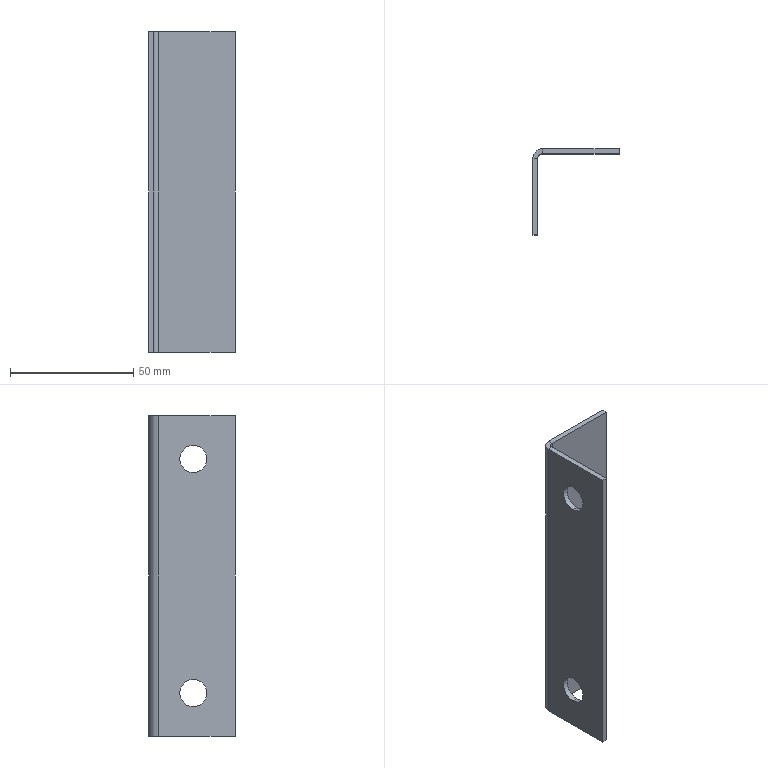Part | SolidWorks | features FlatPattern 1, ICE 1, SMBaseFlange 1, SheetMetal 1 | 1 solid | 18 faces | box 35 x 35 x 130 mm | volume 16965 mm3 | plane 12 | cylinder 6 | commonest cylinder face diameters 11 x4 4 x1 8 x1
STEP:
#1=CARTESIAN_POINT('',(0.,17.,107.));
#2=VERTEX_POINT('',#1);
#3=CARTESIAN_POINT('',(0.,17.,118.));
#4=VERTEX_POINT('',#3);
#5=CARTESIAN_POINT('',(0.,17.,112.5));
#6=DIRECTION('',(-1.,0.,0.));
#7=DIRECTION('',(0.,0.,1.));
#8=AXIS2_PLACEMENT_3D('',#5,#6,#7);
#9=CIRCLE('',#8,5.5);
#10=EDGE_CURVE('',#2,#4,#9,.T.);
#11=ORIENTED_EDGE('',*,*,#10,.T.);
#12=CARTESIAN_POINT('',(2.,17.,118.));
#13=VERTEX_POINT('',#12);
#14=CARTESIAN_POINT('',(-8.,17.,118.));
#15=DIRECTION('',(1.,0.,0.));
#16=VECTOR('',#15,1000.);
#17=LINE('',#14,#16);
#18=EDGE_CURVE('',#4,#13,#17,.T.);
#19=ORIENTED_EDGE('',*,*,#18,.T.);
#20=CARTESIAN_POINT('',(2.,17.,107.));
#21=VERTEX_POINT('',#20);
#22=CARTESIAN_POINT('',(2.,17.,112.5));
#23=DIRECTION('',(1.,0.,0.));
#24=DIRECTION('',(0.,0.,-1.));
#25=AXIS2_PLACEMENT_3D('',#22,#23,#24);
#26=CIRCLE('',#25,5.5);
#27=EDGE_CURVE('',#13,#21,#26,.T.);
#28=ORIENTED_EDGE('',*,*,#27,.T.);
#29=CARTESIAN_POINT('',(-8.,17.,107.));
#30=DIRECTION('',(1.,0.,0.));
#31=VECTOR('',#30,1000.);
#32=LINE('',#29,#31);
#33=EDGE_CURVE('',#2,#21,#32,.T.);
#34=ORIENTED_EDGE('',*,*,#33,.F.);
#35=EDGE_LOOP('',(#11,#19,#28,#34));
#36=FACE_OUTER_BOUND('',#35,.T.);
#37=CARTESIAN_POINT('',(-8.,17.,112.5));
#38=DIRECTION('',(1.,0.,0.));
#39=DIRECTION('',(0.,0.,-1.));
#40=AXIS2_PLACEMENT_3D('',#37,#38,#39);
#41=CYLINDRICAL_SURFACE('',#40,5.5);
#42=ADVANCED_FACE('',(#36),#41,.F.);
#43=CARTESIAN_POINT('',(0.,17.,12.));
#44=VERTEX_POINT('',#43);
#45=CARTESIAN_POINT('',(0.,17.,23.));
#46=VERTEX_POINT('',#45);
#47=CARTESIAN_POINT('',(0.,17.,17.5));
#48=DIRECTION('',(-1.,0.,0.));
#49=DIRECTION('',(0.,0.,1.));
#50=AXIS2_PLACEMENT_3D('',#47,#48,#49);
#51=CIRCLE('',#50,5.5);
#52=EDGE_CURVE('',#44,#46,#51,.T.);
#53=ORIENTED_EDGE('',*,*,#52,.T.);
#54=CARTESIAN_POINT('',(2.,17.,23.));
#55=VERTEX_POINT('',#54);
#56=CARTESIAN_POINT('',(-8.,17.,23.));
#57=DIRECTION('',(1.,0.,0.));
#58=VECTOR('',#57,1000.);
#59=LINE('',#56,#58);
#60=EDGE_CURVE('',#46,#55,#59,.T.);
#61=ORIENTED_EDGE('',*,*,#60,.T.);
#62=CARTESIAN_POINT('',(2.,17.,12.));
#63=VERTEX_POINT('',#62);
#64=CARTESIAN_POINT('',(2.,17.,17.5));
#65=DIRECTION('',(1.,0.,0.));
#66=DIRECTION('',(0.,0.,-1.));
#67=AXIS2_PLACEMENT_3D('',#64,#65,#66);
#68=CIRCLE('',#67,5.5);
#69=EDGE_CURVE('',#55,#63,#68,.T.);
#70=ORIENTED_EDGE('',*,*,#69,.T.);
#71=CARTESIAN_POINT('',(-8.,17.,12.));
#72=DIRECTION('',(1.,0.,0.));
#73=VECTOR('',#72,1000.);
#74=LINE('',#71,#73);
#75=EDGE_CURVE('',#44,#63,#74,.T.);
#76=ORIENTED_EDGE('',*,*,#75,.F.);
#77=EDGE_LOOP('',(#53,#61,#70,#76));
#78=FACE_OUTER_BOUND('',#77,.T.);
#79=CARTESIAN_POINT('',(-8.,17.,17.5));
#80=DIRECTION('',(1.,0.,0.));
#81=DIRECTION('',(0.,0.,-1.));
#82=AXIS2_PLACEMENT_3D('',#79,#80,#81);
#83=CYLINDRICAL_SURFACE('',#82,5.5);
#84=ADVANCED_FACE('',(#78),#83,.F.);
#85=CARTESIAN_POINT('',(4.,35.,130.));
#86=VERTEX_POINT('',#85);
#87=CARTESIAN_POINT('',(4.,33.,130.));
#88=VERTEX_POINT('',#87);
#89=CARTESIAN_POINT('',(4.,35.,130.));
#90=DIRECTION('',(0.,-1.,0.));
#91=VECTOR('',#90,1000.);
#92=LINE('',#89,#91);
#93=EDGE_CURVE('',#86,#88,#92,.T.);
#94=ORIENTED_EDGE('',*,*,#93,.F.);
#95=CARTESIAN_POINT('',(0.,31.,130.));
#96=VERTEX_POINT('',#95);
#97=CARTESIAN_POINT('',(4.,31.,130.));
#98=DIRECTION('',(0.,0.,-1.));
#99=DIRECTION('',(1.,0.,0.));
#100=AXIS2_PLACEMENT_3D('',#97,#98,#99);
#101=CIRCLE('',#100,4.);
#102=EDGE_CURVE('',#96,#86,#101,.T.);
#103=ORIENTED_EDGE('',*,*,#102,.F.);
#104=CARTESIAN_POINT('',(2.,31.,130.));
#105=VERTEX_POINT('',#104);
#106=CARTESIAN_POINT('',(2.,31.,130.));
#107=DIRECTION('',(-1.,0.,0.));
#108=VECTOR('',#107,1000.);
#109=LINE('',#106,#108);
#110=EDGE_CURVE('',#105,#96,#109,.T.);
#111=ORIENTED_EDGE('',*,*,#110,.F.);
#112=CARTESIAN_POINT('',(4.,31.,130.));
#113=DIRECTION('',(0.,0.,-1.));
#114=DIRECTION('',(1.,0.,0.));
#115=AXIS2_PLACEMENT_3D('',#112,#113,#114);
#116=CIRCLE('',#115,2.);
#117=EDGE_CURVE('',#105,#88,#116,.T.);
#118=ORIENTED_EDGE('',*,*,#117,.T.);
#119=EDGE_LOOP('',(#94,#103,#111,#118));
#120=FACE_OUTER_BOUND('',#119,.T.);
#121=CARTESIAN_POINT('',(4.,35.,130.));
#122=DIRECTION('',(0.,0.,1.));
#123=DIRECTION('',(1.,0.,0.));
#124=AXIS2_PLACEMENT_3D('',#121,#122,#123);
#125=PLANE('',#124);
#126=ADVANCED_FACE('',(#120),#125,.T.);
#127=CARTESIAN_POINT('',(35.,35.,130.));
#128=VERTEX_POINT('',#127);
#129=CARTESIAN_POINT('',(0.,35.,130.));
#130=DIRECTION('',(1.,0.,0.));
#131=VECTOR('',#130,1000.);
#132=LINE('',#129,#131);
#133=EDGE_CURVE('',#86,#128,#132,.T.);
#134=ORIENTED_EDGE('',*,*,#133,.F.);
#135=ORIENTED_EDGE('',*,*,#93,.T.);
#136=CARTESIAN_POINT('',(35.,33.,130.));
#137=VERTEX_POINT('',#136);
#138=CARTESIAN_POINT('',(0.,33.,130.));
#139=DIRECTION('',(1.,0.,0.));
#140=VECTOR('',#139,1000.);
#141=LINE('',#138,#140);
#142=EDGE_CURVE('',#88,#137,#141,.T.);
#143=ORIENTED_EDGE('',*,*,#142,.T.);
#144=CARTESIAN_POINT('',(35.,35.,130.));
#145=DIRECTION('',(0.,-1.,0.));
#146=VECTOR('',#145,1000.);
#147=LINE('',#144,#146);
#148=EDGE_CURVE('',#128,#137,#147,.T.);
#149=ORIENTED_EDGE('',*,*,#148,.F.);
#150=EDGE_LOOP('',(#134,#135,#143,#149));
#151=FACE_OUTER_BOUND('',#150,.T.);
#152=CARTESIAN_POINT('',(2.,31.,130.));
#153=DIRECTION('',(0.,0.,1.));
#154=DIRECTION('',(1.,0.,0.));
#155=AXIS2_PLACEMENT_3D('',#152,#153,#154);
#156=PLANE('',#155);
#157=ADVANCED_FACE('',(#151),#156,.T.);
#158=CARTESIAN_POINT('',(0.,31.,0.));
#159=VERTEX_POINT('',#158);
#160=CARTESIAN_POINT('',(2.,31.,0.));
#161=VERTEX_POINT('',#160);
#162=CARTESIAN_POINT('',(0.,31.,0.));
#163=DIRECTION('',(1.,0.,0.));
#164=VECTOR('',#163,1000.);
#165=LINE('',#162,#164);
#166=EDGE_CURVE('',#159,#161,#165,.T.);
#167=ORIENTED_EDGE('',*,*,#166,.F.);
#168=CARTESIAN_POINT('',(4.,35.,0.));
#169=VERTEX_POINT('',#168);
#170=CARTESIAN_POINT('',(4.,31.,0.));
#171=DIRECTION('',(0.,0.,-1.));
#172=DIRECTION('',(1.,0.,0.));
#173=AXIS2_PLACEMENT_3D('',#170,#171,#172);
#174=CIRCLE('',#173,4.);
#175=EDGE_CURVE('',#159,#169,#174,.T.);
#176=ORIENTED_EDGE('',*,*,#175,.T.);
#177=CARTESIAN_POINT('',(4.,33.,0.));
#178=VERTEX_POINT('',#177);
#179=CARTESIAN_POINT('',(4.,33.,0.));
#180=DIRECTION('',(0.,1.,0.));
#181=VECTOR('',#180,1000.);
#182=LINE('',#179,#181);
#183=EDGE_CURVE('',#178,#169,#182,.T.);
#184=ORIENTED_EDGE('',*,*,#183,.F.);
#185=CARTESIAN_POINT('',(4.,31.,0.));
#186=DIRECTION('',(0.,0.,-1.));
#187=DIRECTION('',(1.,0.,0.));
#188=AXIS2_PLACEMENT_3D('',#185,#186,#187);
#189=CIRCLE('',#188,2.);
#190=EDGE_CURVE('',#161,#178,#189,.T.);
#191=ORIENTED_EDGE('',*,*,#190,.F.);
#192=EDGE_LOOP('',(#167,#176,#184,#191));
#193=FACE_OUTER_BOUND('',#192,.T.);
#194=CARTESIAN_POINT('',(0.,31.,0.));
#195=DIRECTION('',(0.,0.,-1.));
#196=DIRECTION('',(-1.,0.,0.));
#197=AXIS2_PLACEMENT_3D('',#194,#195,#196);
#198=PLANE('',#197);
#199=ADVANCED_FACE('',(#193),#198,.T.);
#200=CARTESIAN_POINT('',(0.,0.,0.));
#201=VERTEX_POINT('',#200);
#202=CARTESIAN_POINT('',(0.,0.,0.));
#203=DIRECTION('',(0.,1.,0.));
#204=VECTOR('',#203,1000.);
#205=LINE('',#202,#204);
#206=EDGE_CURVE('',#201,#159,#205,.T.);
#207=ORIENTED_EDGE('',*,*,#206,.T.);
#208=ORIENTED_EDGE('',*,*,#166,.T.);
#209=CARTESIAN_POINT('',(2.,0.,0.));
#210=VERTEX_POINT('',#209);
#211=CARTESIAN_POINT('',(2.,0.,0.));
#212=DIRECTION('',(0.,1.,0.));
#213=VECTOR('',#212,1000.);
#214=LINE('',#211,#213);
#215=EDGE_CURVE('',#210,#161,#214,.T.);
#216=ORIENTED_EDGE('',*,*,#215,.F.);
#217=CARTESIAN_POINT('',(2.,0.,0.));
#218=DIRECTION('',(-1.,0.,0.));
#219=VECTOR('',#218,1000.);
#220=LINE('',#217,#219);
#221=EDGE_CURVE('',#210,#201,#220,.T.);
#222=ORIENTED_EDGE('',*,*,#221,.T.);
#223=EDGE_LOOP('',(#207,#208,#216,#222));
#224=FACE_OUTER_BOUND('',#223,.T.);
#225=CARTESIAN_POINT('',(4.,33.,0.));
#226=DIRECTION('',(0.,0.,-1.));
#227=DIRECTION('',(-1.,0.,0.));
#228=AXIS2_PLACEMENT_3D('',#225,#226,#227);
#229=PLANE('',#228);
#230=ADVANCED_FACE('',(#224),#229,.T.);
#231=CARTESIAN_POINT('',(35.,33.,0.));
#232=VERTEX_POINT('',#231);
#233=CARTESIAN_POINT('',(0.,33.,0.));
#234=DIRECTION('',(1.,0.,0.));
#235=VECTOR('',#234,1000.);
#236=LINE('',#233,#235);
#237=EDGE_CURVE('',#178,#232,#236,.T.);
#238=ORIENTED_EDGE('',*,*,#237,.T.);
#239=CARTESIAN_POINT('',(35.,33.,130.));
#240=DIRECTION('',(0.,0.,-1.));
#241=VECTOR('',#240,1000.);
#242=LINE('',#239,#241);
#243=EDGE_CURVE('',#137,#232,#242,.T.);
#244=ORIENTED_EDGE('',*,*,#243,.F.);
#245=ORIENTED_EDGE('',*,*,#142,.F.);
#246=CARTESIAN_POINT('',(4.,33.,130.));
#247=DIRECTION('',(0.,0.,-1.));
#248=VECTOR('',#247,1000.);
#249=LINE('',#246,#248);
#250=EDGE_CURVE('',#88,#178,#249,.T.);
#251=ORIENTED_EDGE('',*,*,#250,.T.);
#252=EDGE_LOOP('',(#238,#244,#245,#251));
#253=FACE_OUTER_BOUND('',#252,.T.);
#254=CARTESIAN_POINT('',(0.,33.,130.));
#255=DIRECTION('',(0.,1.,0.));
#256=DIRECTION('',(0.,0.,1.));
#257=AXIS2_PLACEMENT_3D('',#254,#255,#256);
#258=PLANE('',#257);
#259=ADVANCED_FACE('',(#253),#258,.F.);
#260=CARTESIAN_POINT('',(35.,35.,0.));
#261=VERTEX_POINT('',#260);
#262=CARTESIAN_POINT('',(35.,35.,0.));
#263=DIRECTION('',(0.,-1.,0.));
#264=VECTOR('',#263,1000.);
#265=LINE('',#262,#264);
#266=EDGE_CURVE('',#261,#232,#265,.T.);
#267=ORIENTED_EDGE('',*,*,#266,.F.);
#268=CARTESIAN_POINT('',(35.,35.,130.));
#269=DIRECTION('',(0.,0.,-1.));
#270=VECTOR('',#269,1000.);
#271=LINE('',#268,#270);
#272=EDGE_CURVE('',#128,#261,#271,.T.);
#273=ORIENTED_EDGE('',*,*,#272,.F.);
#274=ORIENTED_EDGE('',*,*,#148,.T.);
#275=ORIENTED_EDGE('',*,*,#243,.T.);
#276=EDGE_LOOP('',(#267,#273,#274,#275));
#277=FACE_OUTER_BOUND('',#276,.T.);
#278=CARTESIAN_POINT('',(35.,35.,130.));
#279=DIRECTION('',(1.,0.,0.));
#280=DIRECTION('',(0.,0.,-1.));
#281=AXIS2_PLACEMENT_3D('',#278,#279,#280);
#282=PLANE('',#281);
#283=ADVANCED_FACE('',(#277),#282,.T.);
#284=CARTESIAN_POINT('',(0.,35.,0.));
#285=DIRECTION('',(1.,0.,0.));
#286=VECTOR('',#285,1000.);
#287=LINE('',#284,#286);
#288=EDGE_CURVE('',#169,#261,#287,.T.);
#289=ORIENTED_EDGE('',*,*,#288,.F.);
#290=CARTESIAN_POINT('',(4.,35.,130.));
#291=DIRECTION('',(0.,0.,-1.));
#292=VECTOR('',#291,1000.);
#293=LINE('',#290,#292);
#294=EDGE_CURVE('',#86,#169,#293,.T.);
#295=ORIENTED_EDGE('',*,*,#294,.F.);
#296=ORIENTED_EDGE('',*,*,#133,.T.);
#297=ORIENTED_EDGE('',*,*,#272,.T.);
#298=EDGE_LOOP('',(#289,#295,#296,#297));
#299=FACE_OUTER_BOUND('',#298,.T.);
#300=CARTESIAN_POINT('',(0.,35.,130.));
#301=DIRECTION('',(0.,1.,0.));
#302=DIRECTION('',(0.,0.,1.));
#303=AXIS2_PLACEMENT_3D('',#300,#301,#302);
#304=PLANE('',#303);
#305=ADVANCED_FACE('',(#299),#304,.T.);
#306=ORIENTED_EDGE('',*,*,#175,.F.);
#307=CARTESIAN_POINT('',(0.,31.,130.));
#308=DIRECTION('',(0.,0.,-1.));
#309=VECTOR('',#308,1000.);
#310=LINE('',#307,#309);
#311=EDGE_CURVE('',#96,#159,#310,.T.);
#312=ORIENTED_EDGE('',*,*,#311,.F.);
#313=ORIENTED_EDGE('',*,*,#102,.T.);
#314=ORIENTED_EDGE('',*,*,#294,.T.);
#315=EDGE_LOOP('',(#306,#312,#313,#314));
#316=FACE_OUTER_BOUND('',#315,.T.);
#317=CARTESIAN_POINT('',(4.,31.,130.));
#318=DIRECTION('',(0.,0.,-1.));
#319=DIRECTION('',(-1.,0.,0.));
#320=AXIS2_PLACEMENT_3D('',#317,#318,#319);
#321=CYLINDRICAL_SURFACE('',#320,4.);
#322=ADVANCED_FACE('',(#316),#321,.T.);
#323=ORIENTED_EDGE('',*,*,#10,.F.);
#324=CARTESIAN_POINT('',(0.,17.,112.5));
#325=DIRECTION('',(-1.,0.,0.));
#326=DIRECTION('',(0.,0.,1.));
#327=AXIS2_PLACEMENT_3D('',#324,#325,#326);
#328=CIRCLE('',#327,5.5);
#329=EDGE_CURVE('',#4,#2,#328,.T.);
#330=ORIENTED_EDGE('',*,*,#329,.F.);
#331=EDGE_LOOP('',(#323,#330));
#332=FACE_BOUND('',#331,.T.);
#333=ORIENTED_EDGE('',*,*,#52,.F.);
#334=CARTESIAN_POINT('',(0.,17.,17.5));
#335=DIRECTION('',(-1.,0.,0.));
#336=DIRECTION('',(0.,0.,1.));
#337=AXIS2_PLACEMENT_3D('',#334,#335,#336);
#338=CIRCLE('',#337,5.5);
#339=EDGE_CURVE('',#46,#44,#338,.T.);
#340=ORIENTED_EDGE('',*,*,#339,.F.);
#341=EDGE_LOOP('',(#333,#340));
#342=FACE_BOUND('',#341,.T.);
#343=ORIENTED_EDGE('',*,*,#206,.F.);
#344=CARTESIAN_POINT('',(0.,0.,130.));
#345=VERTEX_POINT('',#344);
#346=CARTESIAN_POINT('',(0.,0.,130.));
#347=DIRECTION('',(0.,0.,-1.));
#348=VECTOR('',#347,1000.);
#349=LINE('',#346,#348);
#350=EDGE_CURVE('',#345,#201,#349,.T.);
#351=ORIENTED_EDGE('',*,*,#350,.F.);
#352=CARTESIAN_POINT('',(0.,0.,130.));
#353=DIRECTION('',(0.,1.,0.));
#354=VECTOR('',#353,1000.);
#355=LINE('',#352,#354);
#356=EDGE_CURVE('',#345,#96,#355,.T.);
#357=ORIENTED_EDGE('',*,*,#356,.T.);
#358=ORIENTED_EDGE('',*,*,#311,.T.);
#359=EDGE_LOOP('',(#343,#351,#357,#358));
#360=FACE_OUTER_BOUND('',#359,.T.);
#361=CARTESIAN_POINT('',(0.,0.,130.));
#362=DIRECTION('',(-1.,0.,0.));
#363=DIRECTION('',(0.,0.,1.));
#364=AXIS2_PLACEMENT_3D('',#361,#362,#363);
#365=PLANE('',#364);
#366=ADVANCED_FACE('',(#332,#342,#360),#365,.T.);
#367=ORIENTED_EDGE('',*,*,#221,.F.);
#368=CARTESIAN_POINT('',(2.,0.,130.));
#369=VERTEX_POINT('',#368);
#370=CARTESIAN_POINT('',(2.,0.,130.));
#371=DIRECTION('',(0.,0.,-1.));
#372=VECTOR('',#371,1000.);
#373=LINE('',#370,#372);
#374=EDGE_CURVE('',#369,#210,#373,.T.);
#375=ORIENTED_EDGE('',*,*,#374,.F.);
#376=CARTESIAN_POINT('',(2.,0.,130.));
#377=DIRECTION('',(-1.,0.,0.));
#378=VECTOR('',#377,1000.);
#379=LINE('',#376,#378);
#380=EDGE_CURVE('',#369,#345,#379,.T.);
#381=ORIENTED_EDGE('',*,*,#380,.T.);
#382=ORIENTED_EDGE('',*,*,#350,.T.);
#383=EDGE_LOOP('',(#367,#375,#381,#382));
#384=FACE_OUTER_BOUND('',#383,.T.);
#385=CARTESIAN_POINT('',(2.,0.,130.));
#386=DIRECTION('',(0.,-1.,0.));
#387=DIRECTION('',(0.,0.,-1.));
#388=AXIS2_PLACEMENT_3D('',#385,#386,#387);
#389=PLANE('',#388);
#390=ADVANCED_FACE('',(#384),#389,.T.);
#391=CARTESIAN_POINT('',(2.,17.,112.5));
#392=DIRECTION('',(1.,0.,0.));
#393=DIRECTION('',(0.,0.,-1.));
#394=AXIS2_PLACEMENT_3D('',#391,#392,#393);
#395=CIRCLE('',#394,5.5);
#396=EDGE_CURVE('',#21,#13,#395,.T.);
#397=ORIENTED_EDGE('',*,*,#396,.F.);
#398=ORIENTED_EDGE('',*,*,#27,.F.);
#399=EDGE_LOOP('',(#397,#398));
#400=FACE_BOUND('',#399,.T.);
#401=CARTESIAN_POINT('',(2.,17.,17.5));
#402=DIRECTION('',(1.,0.,0.));
#403=DIRECTION('',(0.,0.,-1.));
#404=AXIS2_PLACEMENT_3D('',#401,#402,#403);
#405=CIRCLE('',#404,5.5);
#406=EDGE_CURVE('',#63,#55,#405,.T.);
#407=ORIENTED_EDGE('',*,*,#406,.F.);
#408=ORIENTED_EDGE('',*,*,#69,.F.);
#409=EDGE_LOOP('',(#407,#408));
#410=FACE_BOUND('',#409,.T.);
#411=ORIENTED_EDGE('',*,*,#215,.T.);
#412=CARTESIAN_POINT('',(2.,31.,130.));
#413=DIRECTION('',(0.,0.,-1.));
#414=VECTOR('',#413,1000.);
#415=LINE('',#412,#414);
#416=EDGE_CURVE('',#105,#161,#415,.T.);
#417=ORIENTED_EDGE('',*,*,#416,.F.);
#418=CARTESIAN_POINT('',(2.,0.,130.));
#419=DIRECTION('',(0.,1.,0.));
#420=VECTOR('',#419,1000.);
#421=LINE('',#418,#420);
#422=EDGE_CURVE('',#369,#105,#421,.T.);
#423=ORIENTED_EDGE('',*,*,#422,.F.);
#424=ORIENTED_EDGE('',*,*,#374,.T.);
#425=EDGE_LOOP('',(#411,#417,#423,#424));
#426=FACE_OUTER_BOUND('',#425,.T.);
#427=CARTESIAN_POINT('',(2.,0.,130.));
#428=DIRECTION('',(-1.,0.,0.));
#429=DIRECTION('',(0.,0.,1.));
#430=AXIS2_PLACEMENT_3D('',#427,#428,#429);
#431=PLANE('',#430);
#432=ADVANCED_FACE('',(#400,#410,#426),#431,.F.);
#433=ORIENTED_EDGE('',*,*,#190,.T.);
#434=ORIENTED_EDGE('',*,*,#250,.F.);
#435=ORIENTED_EDGE('',*,*,#117,.F.);
#436=ORIENTED_EDGE('',*,*,#416,.T.);
#437=EDGE_LOOP('',(#433,#434,#435,#436));
#438=FACE_OUTER_BOUND('',#437,.T.);
#439=CARTESIAN_POINT('',(4.,31.,130.));
#440=DIRECTION('',(0.,0.,-1.));
#441=DIRECTION('',(-1.,0.,0.));
#442=AXIS2_PLACEMENT_3D('',#439,#440,#441);
#443=CYLINDRICAL_SURFACE('',#442,2.);
#444=ADVANCED_FACE('',(#438),#443,.F.);
#445=ORIENTED_EDGE('',*,*,#422,.T.);
#446=ORIENTED_EDGE('',*,*,#110,.T.);
#447=ORIENTED_EDGE('',*,*,#356,.F.);
#448=ORIENTED_EDGE('',*,*,#380,.F.);
#449=EDGE_LOOP('',(#445,#446,#447,#448));
#450=FACE_OUTER_BOUND('',#449,.T.);
#451=CARTESIAN_POINT('',(4.,31.,130.));
#452=DIRECTION('',(0.,0.,1.));
#453=DIRECTION('',(1.,0.,0.));
#454=AXIS2_PLACEMENT_3D('',#451,#452,#453);
#455=PLANE('',#454);
#456=ADVANCED_FACE('',(#450),#455,.T.);
#457=ORIENTED_EDGE('',*,*,#237,.F.);
#458=ORIENTED_EDGE('',*,*,#183,.T.);
#459=ORIENTED_EDGE('',*,*,#288,.T.);
#460=ORIENTED_EDGE('',*,*,#266,.T.);
#461=EDGE_LOOP('',(#457,#458,#459,#460));
#462=FACE_OUTER_BOUND('',#461,.T.);
#463=CARTESIAN_POINT('',(4.,31.,0.));
#464=DIRECTION('',(0.,0.,1.));
#465=DIRECTION('',(1.,0.,0.));
#466=AXIS2_PLACEMENT_3D('',#463,#464,#465);
#467=PLANE('',#466);
#468=ADVANCED_FACE('',(#462),#467,.F.);
#469=ORIENTED_EDGE('',*,*,#60,.F.);
#470=ORIENTED_EDGE('',*,*,#339,.T.);
#471=ORIENTED_EDGE('',*,*,#75,.T.);
#472=ORIENTED_EDGE('',*,*,#406,.T.);
#473=EDGE_LOOP('',(#469,#470,#471,#472));
#474=FACE_OUTER_BOUND('',#473,.T.);
#475=CARTESIAN_POINT('',(-8.,17.,17.5));
#476=DIRECTION('',(1.,0.,0.));
#477=DIRECTION('',(0.,0.,-1.));
#478=AXIS2_PLACEMENT_3D('',#475,#476,#477);
#479=CYLINDRICAL_SURFACE('',#478,5.5);
#480=ADVANCED_FACE('',(#474),#479,.F.);
#481=ORIENTED_EDGE('',*,*,#18,.F.);
#482=ORIENTED_EDGE('',*,*,#329,.T.);
#483=ORIENTED_EDGE('',*,*,#33,.T.);
#484=ORIENTED_EDGE('',*,*,#396,.T.);
#485=EDGE_LOOP('',(#481,#482,#483,#484));
#486=FACE_OUTER_BOUND('',#485,.T.);
#487=CARTESIAN_POINT('',(-8.,17.,112.5));
#488=DIRECTION('',(1.,0.,0.));
#489=DIRECTION('',(0.,0.,-1.));
#490=AXIS2_PLACEMENT_3D('',#487,#488,#489);
#491=CYLINDRICAL_SURFACE('',#490,5.5);
#492=ADVANCED_FACE('',(#486),#491,.F.);
#493=CLOSED_SHELL('',(#42,#84,#126,#157,#199,#230,#259,#283,#305,#322,#366,#390,#432,#444,#456,#468,#480,#492));
#494=MANIFOLD_SOLID_BREP('',#493);
#495=CARTESIAN_POINT('',(0.,0.,0.));
#496=DIRECTION('',(0.,0.,1.));
#497=DIRECTION('',(1.,0.,0.));
#498=AXIS2_PLACEMENT_3D('',#495,#496,#497);
#499=(LENGTH_UNIT()NAMED_UNIT(*)SI_UNIT(.MILLI.,.METRE.));
#500=UNCERTAINTY_MEASURE_WITH_UNIT(LENGTH_MEASURE(0.00001),#499,'','');
#501=(NAMED_UNIT(*)PLANE_ANGLE_UNIT()SI_UNIT($,.RADIAN.));
#502=(NAMED_UNIT(*)SI_UNIT($,.STERADIAN.)SOLID_ANGLE_UNIT());
#503=(GEOMETRIC_REPRESENTATION_CONTEXT(3)GLOBAL_UNCERTAINTY_ASSIGNED_CONTEXT((#500))GLOBAL_UNIT_ASSIGNED_CONTEXT((#499,#501,#502))REPRESENTATION_CONTEXT('',''));
#504=ADVANCED_BREP_SHAPE_REPRESENTATION('',(#494,#498),#503);